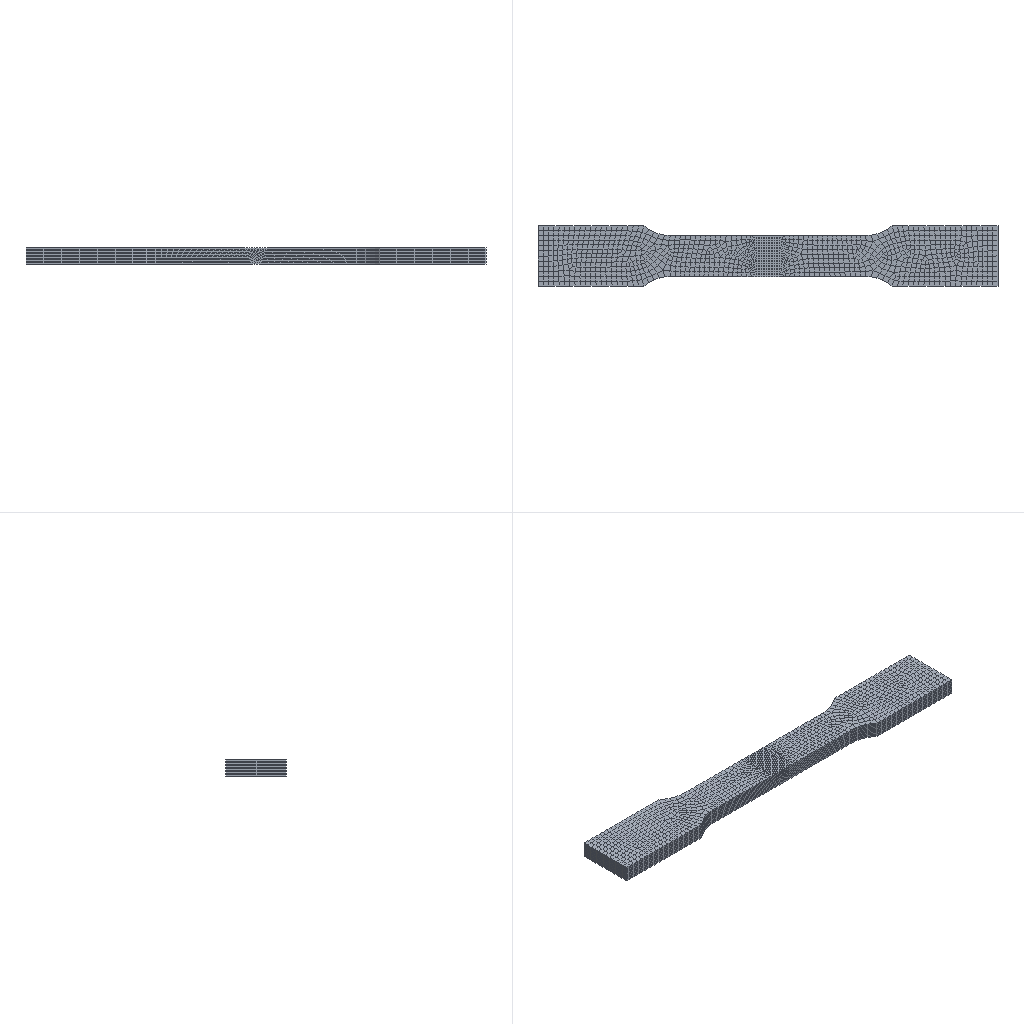Simulation study | abaqus
Set-up summary:
category,name,step,type,value,unit,region
solver,abaqus
solver,version,,,Abaqus/Explicit 3DEXPERIENCE R2017x
units,not stated in the deck,,not stated
analysis,deck,,transient,transient
load_step,Step-1,Step-1,transient,nlgeom=True
contact,interactions,,,general=0 pairs=0 ties=0
load_step,requested,,,1
mesh,nodes,,,18008
mesh,elements,,,15338
element_type,C3D8RT,,solid,15338
load,load commands in deck,,count,1
bc,support commands in deck,,count,7
material,MATERIAL-1,,in results
material,MATERIAL-1-NO,,in results
check,setup vs results,,match,"per instance, exact: element labels, types and connectivity; labels of the nodes the elements use; coordinates of those nodes at SINGLE_PRECISION in 1 of 1 instance(s)"
Abaqus input file, long lists of numbers shortened:
*Heading
** Job name: Job-2 Model name: Model-1-Copy
** Generated by: Abaqus/CAE 2017
*Preprint, echo=NO, model=NO, history=NO, contact=NO
**
** PARTS
**
*Part, name=work
*Node
      1,  -7.129,   4.899, 0.01586
      2,  -2.993,   4.901,         -10.
** (18006 more lines like these left out)
*Element, type=C3D8RT
    1,    93,    94,   837,   857,  1160,  1161,  6009,  6029
    2,   837,    57,    58,   873,  6009,  1109,  1110,  6045
** (15336 more lines like these left out)
*Nset, nset=SET-4, generate
     1,  18008,      1
*Elset, elset=SET-4, generate
     1,  15338,      1
*Elset, elset=Set-2
     1,     2,     3,     4,     5,     6,     7,     8,     9,    10,    11,    12,    13,    14,    15,    16
    17,    18,    19,    20,    21,    22,    23,    24,    25,    26,    27,    28,    29,    30,    31,    32
** (264 more lines like these left out)
*Elset, elset=Set-3
  3157,  3158,  3159,  3160,  3161,  3162,  3163,  3164,  3165,  3169,  3186,  3188,  3190,  3191,  3192,  3193
  3194,  3195,  3196,  3197,  3198,  3199,  3200,  3201,  3202,  3203,  3204,  3205,  3206,  3207,  3208,  3209
** (691 more lines like these left out)
** Section: Section-1
*Solid Section, elset=Set-2, material=Material-1
,
** Section: Section-2
*Solid Section, elset=Set-3, material=Material-1-no
,
*End Part
**
**
** ASSEMBLY
**
*Assembly, name=Assembly
**
*Instance, name=work-1, part=work
          0.,         12.5,         -10.
*End Instance
**
*Node
      1,       141.25,   25.,  -14.537
*Elset, elset=Set-10, instance=work-1, generate
     1,  15338,      1
*Nset, nset=Set-11, instance=work-1
   45,   46,   47,   52,   53,   54,  639,  640,  641,  642,  643,  644,  645,  646,  647,  648
  748,  749,  750,  751,  752,  753,  754,  755,  756,  757,  758,  759,  760,  761,  762,  763
** (8 more lines like these left out)
*Nset, nset=Set-13
 1,
*Nset, nset=m_Set-12
 1,
*Elset, elset=_s_Surf-4_S4, internal, instance=work-1
 3216, 3217, 3221, 3225, 3312, 3766, 3767, 3771, 3775, 3862, 4316, 4317, 4321, 4325, 4412, 4866
 4867, 4871, 4875, 4962, 5416, 5417, 5421, 5425, 5512, 5966, 5967, 5971, 5975, 6062, 6516, 6517
** (2 more lines like these left out)
*Elset, elset=_s_Surf-4_S6, internal, instance=work-1
 3211, 3213, 3214, 3222, 3223, 3313, 3335, 3761, 3763, 3764, 3772, 3773, 3863, 3885, 4311, 4313
 4314, 4322, 4323, 4413, 4435, 4861, 4863, 4864, 4872, 4873, 4963, 4985, 5411, 5413, 5414, 5422
** (3 more lines like these left out)
*Surface, type=ELEMENT, name=s_Surf-4
_s_Surf-4_S4, S4
_s_Surf-4_S6, S6
** Constraint: Constraint-1
*Coupling, constraint name=Constraint-1, ref node=m_Set-12, surface=s_Surf-4
*Kinematic
*End Assembly
*Amplitude, name=Amp-1
             0.,              0.,             0.1,              1.
**
** MATERIALS
**
*Material, name=Material-1
*Conductivity
35.,  25.
36., 100.
38., 250.
26., 500.
26., 750.
29.,1000.
*Damage Initiation, criterion=DUCTILE
 0.3,0.,0.
*Damage Evolution, type=DISPLACEMENT
 0.001,
*Density
 7.8e-09,
*Elastic
208170., 0.29,  25.
204839., 0.29, 100.
195445.,  0.3, 250.
159029., 0.32, 500.
130676., 0.34, 750.
105212., 0.35,1000.
*Expansion
 1.2e-05,
*Plastic
355.,0.
*Specific Heat
   4.6e+08,  25.
   4.8e+08, 100.
  5.53e+08, 250.
 1.185e+09, 500.
  5.93e+08, 750.
  6.27e+08,1000.
*Material, name=Material-1-no
*Conductivity
35.,  25.
36., 100.
38., 250.
26., 500.
26., 750.
29.,1000.
*Density
 7.8e-09,
*Elastic
208170., 0.29,  25.
204839., 0.29, 100.
195445.,  0.3, 250.
159029., 0.32, 500.
130676., 0.34, 750.
105212., 0.35,1000.
*Expansion
 1.2e-05,
*Specific Heat
   4.6e+08,  25.
   4.8e+08, 100.
  5.53e+08, 250.
 1.185e+09, 500.
  5.93e+08, 750.
  6.27e+08,1000.
**
** PHYSICAL CONSTANTS
**
*Physical Constants, absolute zero=-273., stefan boltzmann=5.67e-08
**
** PREDEFINED FIELDS
**
** Name: Predefined Field-1   Type: Stress
*Initial Conditions, type=STRESS, file=F:/temp/Job-1.odb, step=9, inc=38
** ----------------------------------------------------------------
**
** STEP: Step-1
**
*Step, name=Step-1, nlgeom=YES
*Dynamic, Explicit
, 0.1
*Bulk Viscosity
0.06, 1.2
**
** BOUNDARY CONDITIONS
**
** Name: BC-1 Type: 对称/反对称/完全固定
*Boundary
Set-11, ENCASTRE
** Name: [REDACTED] : Displacement/rotation angle
*Boundary, amplitude=Amp-1
Set-13, 1, 1, 5.
Set-13, 2, 2
Set-13, 3, 3
Set-13, 4, 4
Set-13, 5, 5
Set-13, 6, 6
**
** OUTPUT REQUESTS
**
*Restart, write, number interval=1, time marks=NO
**
** FIELD OUTPUT: F-Output-1
**
*Output, field, number interval=30
*Node Output
CF, RF, RM, RT, U, V
*Element Output, directions=YES
E, LE, MISES, MISESMAX, MISESONLY, NE, PE, PEEQ, PEEQMAX, PEEQT, PEMAG, PRESSONLY, S, SDV, SSAVG, STATUS
TEMP, TSHR, VEEQ
*Contact Output
CDISP, CFORCE, CSTRESS
**
** HISTORY OUTPUT: H-Output-1
**
*Output, history, time interval=2e-06
*Node Output, nset=Set-13
RF1, U1
*End Step
Results summary:
result,step,Step-1,completed,increments=1027862 time=0.1/0.1
result,analysis,,,transient
result,last_loadstep,,,1
result,analysis steps,,count,1
result,primary field,,,U
result,reaction total,,FX,247.837,model units
result,reaction total,,FY,30.894,model units
result,reaction total,,FZ,-118.616,model units